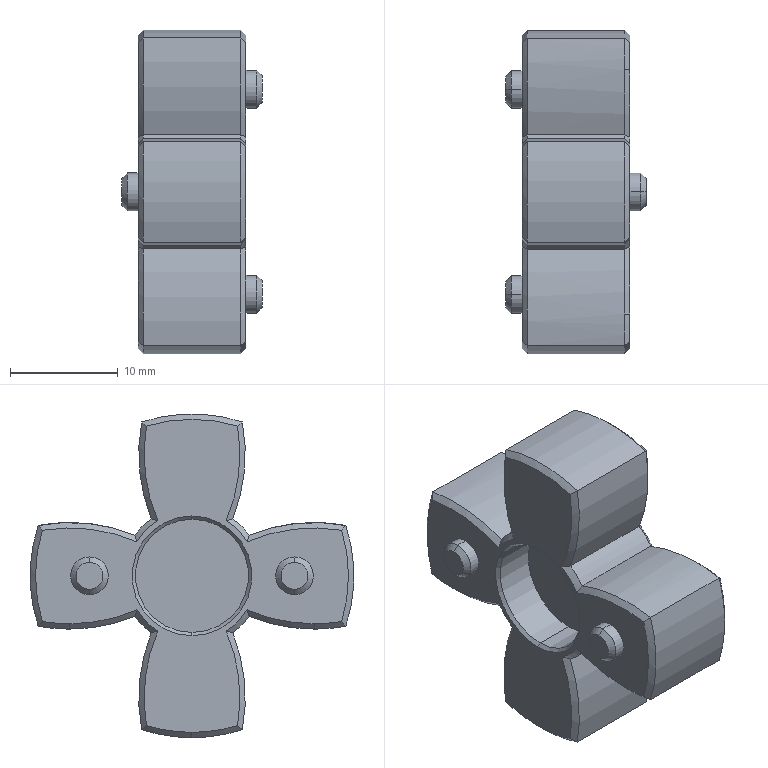Part | NX | features BREP 1 | 1 solid | 88 faces | box 13 x 30 x 30 mm | volume 3929 mm3 | cone 49 | cylinder 31 | plane 8 | commonest cylinder face diameters 32.5 x10 3.5 x8 30 x5 10.5 x4 13 x4